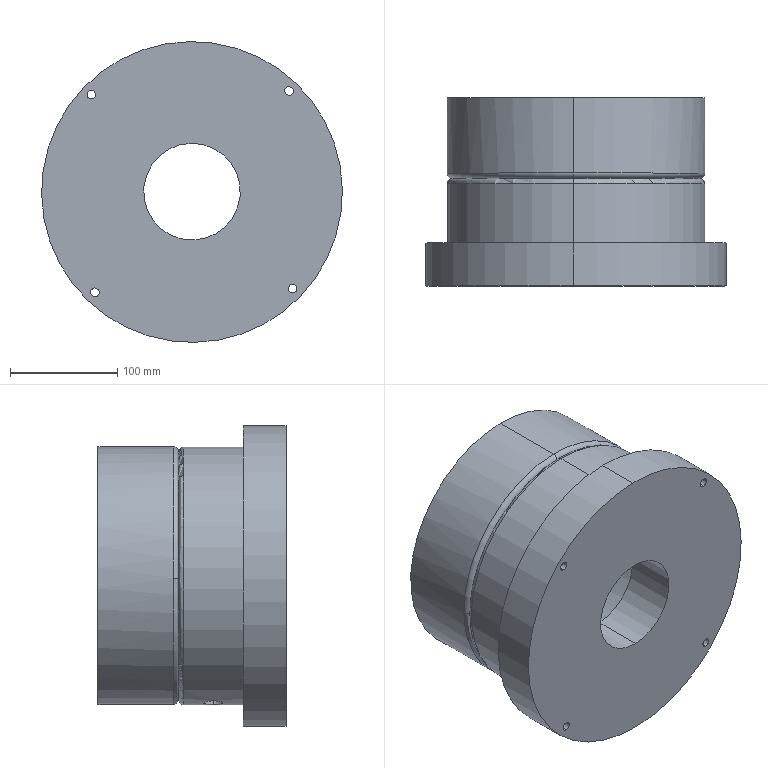Part | STEP file | 2026.6.15-Main Assembly图.sldasm-Part-3 | 1 solid | 70 faces | box 280 x 175 x 280 mm | volume 4284474 mm3 | cylinder 36 | plane 29 | torus 4 | spline 1 | commonest cylinder face diameters 8 x8 16 x8 160 x6 18 x4 240 x4 90 x2